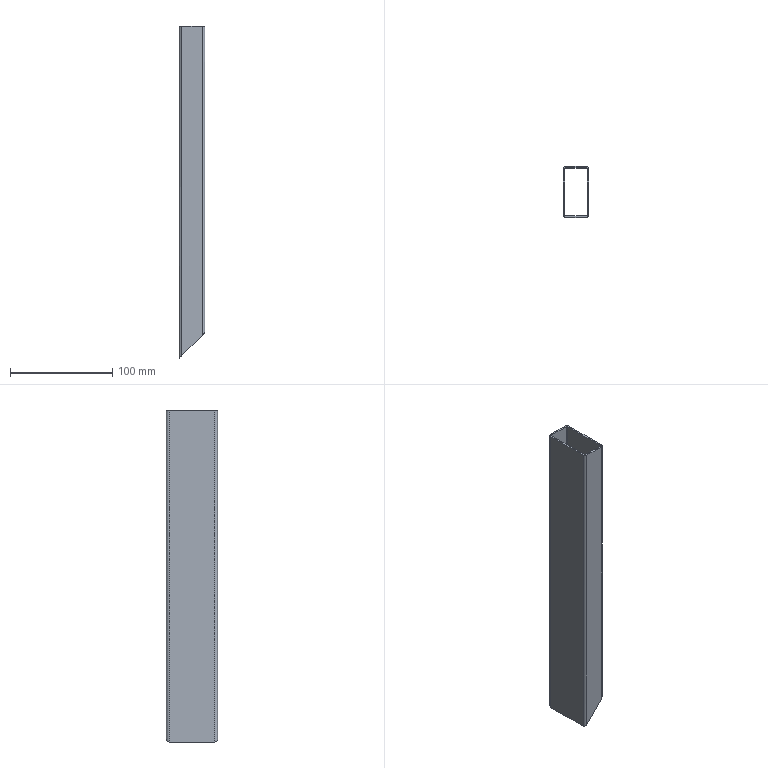Part | STEP file | 7100516 | 1 solid | 19 faces | box 25 x 50 x 325 mm | volume 65710 mm3 | plane 10 | cylinder 9 | commonest cylinder face diameters 2 x4 5 x4 18 x1